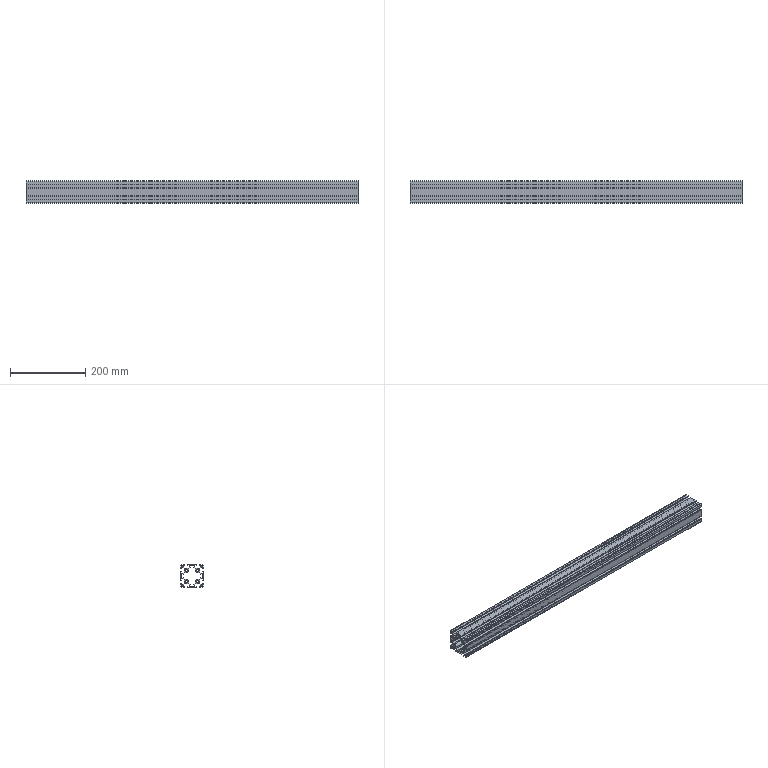Part | STEP file | PN_0014 Lower outer frame front crossbeam_Default <Machined> | 1 solid | 178 faces | box 880 x 60 x 60 mm | volume 809943 mm3 | plane 162 | cylinder 16 | commonest cylinder face diameters 6.8 x8 6.76 x4 11.828 x4